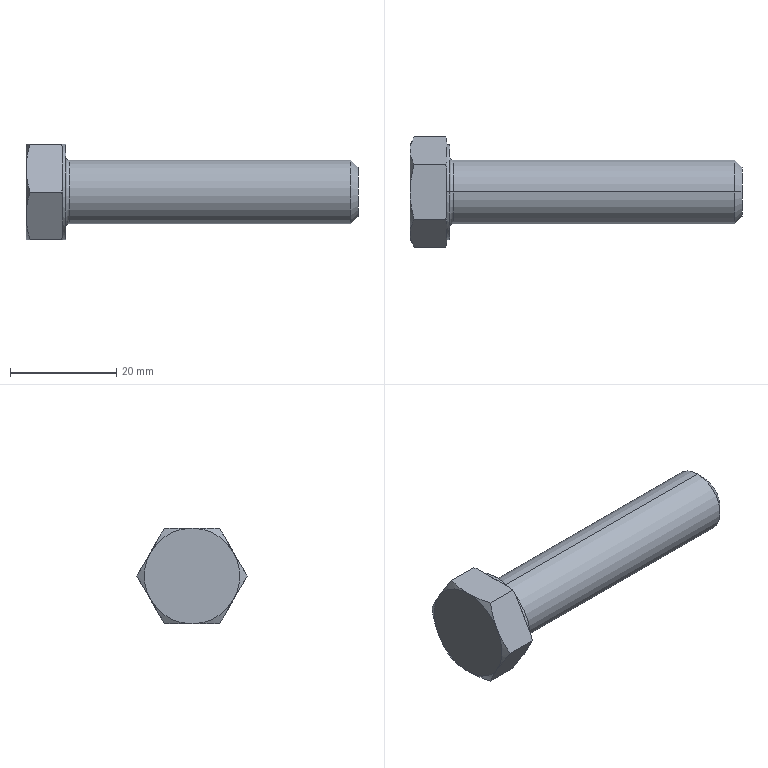Part | SolidWorks | features RevCut 4, Chamfer 1, Extrusion 1, Fillet 1, LPattern 1, Revolution 1 | 1 solid | 35 faces | box 62.5 x 20.785 x 18 mm | volume 8272 mm3 | plane 15 | cone 14 | cylinder 4 | torus 2 | commonest cylinder face diameters 12 x2 18 x2
STEP:
#1=CARTESIAN_POINT('',(8.1,0.,6.));
#2=VERTEX_POINT('',#1);
#3=CARTESIAN_POINT('',(8.1,0.,-6.));
#4=VERTEX_POINT('',#3);
#5=CARTESIAN_POINT('',(8.1,0.,0.));
#6=DIRECTION('',(1.,0.,0.));
#7=DIRECTION('',(0.,0.,-1.));
#8=AXIS2_PLACEMENT_3D('',#5,#6,#7);
#9=CIRCLE('',#8,6.);
#10=EDGE_CURVE('',#2,#4,#9,.T.);
#11=ORIENTED_EDGE('',*,*,#10,.F.);
#12=CARTESIAN_POINT('',(7.5,0.,6.6));
#13=VERTEX_POINT('',#12);
#14=CARTESIAN_POINT('',(8.1,0.,6.6));
#15=DIRECTION('',(0.,1.,0.));
#16=DIRECTION('',(0.,0.,1.));
#17=AXIS2_PLACEMENT_3D('',#14,#15,#16);
#18=CIRCLE('',#17,0.6);
#19=EDGE_CURVE('',#2,#13,#18,.T.);
#20=ORIENTED_EDGE('',*,*,#19,.T.);
#21=CARTESIAN_POINT('',(7.5,0.,-6.6));
#22=VERTEX_POINT('',#21);
#23=CARTESIAN_POINT('',(7.5,0.,0.));
#24=DIRECTION('',(-1.,0.,0.));
#25=DIRECTION('',(0.,0.,-1.));
#26=AXIS2_PLACEMENT_3D('',#23,#24,#25);
#27=CIRCLE('',#26,6.6);
#28=EDGE_CURVE('',#22,#13,#27,.T.);
#29=ORIENTED_EDGE('',*,*,#28,.F.);
#30=CARTESIAN_POINT('',(8.1,0.,-6.6));
#31=DIRECTION('',(0.,-1.,0.));
#32=DIRECTION('',(0.,0.,-1.));
#33=AXIS2_PLACEMENT_3D('',#30,#31,#32);
#34=CIRCLE('',#33,0.6);
#35=EDGE_CURVE('',#4,#22,#34,.T.);
#36=ORIENTED_EDGE('',*,*,#35,.F.);
#37=EDGE_LOOP('',(#11,#20,#29,#36));
#38=FACE_OUTER_BOUND('',#37,.T.);
#39=CARTESIAN_POINT('',(8.1,0.,0.));
#40=DIRECTION('',(1.,0.,0.));
#41=DIRECTION('',(0.,0.,-1.));
#42=AXIS2_PLACEMENT_3D('',#39,#40,#41);
#43=TOROIDAL_SURFACE('',#42,6.6,0.6);
#44=ADVANCED_FACE('',(#38),#43,.F.);
#45=CARTESIAN_POINT('',(62.5,0.,-4.6));
#46=VERTEX_POINT('',#45);
#47=CARTESIAN_POINT('',(62.5,0.,4.6));
#48=VERTEX_POINT('',#47);
#49=CARTESIAN_POINT('',(62.5,0.,0.));
#50=DIRECTION('',(1.,0.,0.));
#51=DIRECTION('',(0.,0.,1.));
#52=AXIS2_PLACEMENT_3D('',#49,#50,#51);
#53=CIRCLE('',#52,4.6);
#54=EDGE_CURVE('',#46,#48,#53,.T.);
#55=ORIENTED_EDGE('',*,*,#54,.F.);
#56=CARTESIAN_POINT('',(61.1,0.,-6.));
#57=VERTEX_POINT('',#56);
#58=CARTESIAN_POINT('',(61.1,0.,-6.));
#59=DIRECTION('',(-0.7071,0.,-0.7071));
#60=VECTOR('',#59,1000.);
#61=LINE('',#58,#60);
#62=EDGE_CURVE('',#46,#57,#61,.T.);
#63=ORIENTED_EDGE('',*,*,#62,.T.);
#64=CARTESIAN_POINT('',(61.1,0.,6.));
#65=VERTEX_POINT('',#64);
#66=CARTESIAN_POINT('',(61.1,0.,0.));
#67=DIRECTION('',(-1.,0.,0.));
#68=DIRECTION('',(0.,0.,1.));
#69=AXIS2_PLACEMENT_3D('',#66,#67,#68);
#70=CIRCLE('',#69,6.);
#71=EDGE_CURVE('',#65,#57,#70,.T.);
#72=ORIENTED_EDGE('',*,*,#71,.F.);
#73=CARTESIAN_POINT('',(61.1,0.,6.));
#74=DIRECTION('',(-0.7071,0.,0.7071));
#75=VECTOR('',#74,1000.);
#76=LINE('',#73,#75);
#77=EDGE_CURVE('',#48,#65,#76,.T.);
#78=ORIENTED_EDGE('',*,*,#77,.F.);
#79=EDGE_LOOP('',(#55,#63,#72,#78));
#80=FACE_OUTER_BOUND('',#79,.T.);
#81=CARTESIAN_POINT('',(61.1,0.,0.));
#82=DIRECTION('',(-1.,0.,0.));
#83=DIRECTION('',(0.,0.,1.));
#84=AXIS2_PLACEMENT_3D('',#81,#82,#83);
#85=CONICAL_SURFACE('',#84,6.,0.7854);
#86=ADVANCED_FACE('',(#80),#85,.T.);
#87=ORIENTED_EDGE('',*,*,#71,.T.);
#88=CARTESIAN_POINT('',(0.,0.,-6.));
#89=DIRECTION('',(-1.,0.,0.));
#90=VECTOR('',#89,1000.);
#91=LINE('',#88,#90);
#92=EDGE_CURVE('',#57,#4,#91,.T.);
#93=ORIENTED_EDGE('',*,*,#92,.T.);
#94=CARTESIAN_POINT('',(8.1,0.,0.));
#95=DIRECTION('',(1.,0.,0.));
#96=DIRECTION('',(0.,0.,-1.));
#97=AXIS2_PLACEMENT_3D('',#94,#95,#96);
#98=CIRCLE('',#97,6.);
#99=EDGE_CURVE('',#4,#2,#98,.T.);
#100=ORIENTED_EDGE('',*,*,#99,.T.);
#101=CARTESIAN_POINT('',(0.,0.,6.));
#102=DIRECTION('',(-1.,0.,0.));
#103=VECTOR('',#102,1000.);
#104=LINE('',#101,#103);
#105=EDGE_CURVE('',#65,#2,#104,.T.);
#106=ORIENTED_EDGE('',*,*,#105,.F.);
#107=EDGE_LOOP('',(#87,#93,#100,#106));
#108=FACE_OUTER_BOUND('',#107,.T.);
#109=CARTESIAN_POINT('',(0.,0.,0.));
#110=DIRECTION('',(-1.,0.,0.));
#111=DIRECTION('',(0.,0.,1.));
#112=AXIS2_PLACEMENT_3D('',#109,#110,#111);
#113=CYLINDRICAL_SURFACE('',#112,6.);
#114=ADVANCED_FACE('',(#108),#113,.T.);
#115=CARTESIAN_POINT('',(7.5,0.,-9.));
#116=VERTEX_POINT('',#115);
#117=CARTESIAN_POINT('',(7.5,0.,9.));
#118=VERTEX_POINT('',#117);
#119=CARTESIAN_POINT('',(7.5,0.,0.));
#120=DIRECTION('',(1.,0.,0.));
#121=DIRECTION('',(0.,0.,-1.));
#122=AXIS2_PLACEMENT_3D('',#119,#120,#121);
#123=CIRCLE('',#122,9.);
#124=EDGE_CURVE('',#116,#118,#123,.T.);
#125=ORIENTED_EDGE('',*,*,#124,.F.);
#126=CARTESIAN_POINT('',(6.9,0.,-9.));
#127=VERTEX_POINT('',#126);
#128=CARTESIAN_POINT('',(0.,0.,-9.));
#129=DIRECTION('',(-1.,0.,0.));
#130=VECTOR('',#129,1000.);
#131=LINE('',#128,#130);
#132=EDGE_CURVE('',#116,#127,#131,.T.);
#133=ORIENTED_EDGE('',*,*,#132,.T.);
#134=CARTESIAN_POINT('',(6.9,7.794,-4.5));
#135=VERTEX_POINT('',#134);
#136=CARTESIAN_POINT('',(6.9,0.,0.));
#137=DIRECTION('',(-1.,0.,0.));
#138=DIRECTION('',(0.,0.,1.));
#139=AXIS2_PLACEMENT_3D('',#136,#137,#138);
#140=CIRCLE('',#139,9.);
#141=EDGE_CURVE('',#135,#127,#140,.T.);
#142=ORIENTED_EDGE('',*,*,#141,.F.);
#143=CARTESIAN_POINT('',(6.9,7.794,4.5));
#144=VERTEX_POINT('',#143);
#145=CARTESIAN_POINT('',(6.9,0.,0.));
#146=DIRECTION('',(-1.,0.,0.));
#147=DIRECTION('',(0.,0.,1.));
#148=AXIS2_PLACEMENT_3D('',#145,#146,#147);
#149=CIRCLE('',#148,9.);
#150=EDGE_CURVE('',#144,#135,#149,.T.);
#151=ORIENTED_EDGE('',*,*,#150,.F.);
#152=CARTESIAN_POINT('',(6.9,0.,9.));
#153=VERTEX_POINT('',#152);
#154=CARTESIAN_POINT('',(6.9,0.,0.));
#155=DIRECTION('',(-1.,0.,0.));
#156=DIRECTION('',(0.,0.,1.));
#157=AXIS2_PLACEMENT_3D('',#154,#155,#156);
#158=CIRCLE('',#157,9.);
#159=EDGE_CURVE('',#153,#144,#158,.T.);
#160=ORIENTED_EDGE('',*,*,#159,.F.);
#161=CARTESIAN_POINT('',(0.,0.,9.));
#162=DIRECTION('',(-1.,0.,0.));
#163=VECTOR('',#162,1000.);
#164=LINE('',#161,#163);
#165=EDGE_CURVE('',#118,#153,#164,.T.);
#166=ORIENTED_EDGE('',*,*,#165,.F.);
#167=EDGE_LOOP('',(#125,#133,#142,#151,#160,#166));
#168=FACE_OUTER_BOUND('',#167,.T.);
#169=CARTESIAN_POINT('',(0.,0.,0.));
#170=DIRECTION('',(-1.,0.,0.));
#171=DIRECTION('',(0.,0.,1.));
#172=AXIS2_PLACEMENT_3D('',#169,#170,#171);
#173=CYLINDRICAL_SURFACE('',#172,9.);
#174=ADVANCED_FACE('',(#168),#173,.T.);
#175=CARTESIAN_POINT('',(6.9,5.57,-8.352));
#176=VERTEX_POINT('',#175);
#177=CARTESIAN_POINT('',(6.9,5.196,-9.));
#178=DIRECTION('',(0.,0.5,0.866));
#179=VECTOR('',#178,1000.);
#180=LINE('',#177,#179);
#181=EDGE_CURVE('',#176,#135,#180,.T.);
#182=ORIENTED_EDGE('',*,*,#181,.F.);
#183=CARTESIAN_POINT('',(6.696,5.196,-9.));
#184=VERTEX_POINT('',#183);
#185=CARTESIAN_POINT('',(6.696,5.196,-9.));
#186=CARTESIAN_POINT('',(6.768,5.321,-8.785));
#187=CARTESIAN_POINT('',(6.836,5.445,-8.569));
#188=CARTESIAN_POINT('',(6.9,5.57,-8.352));
#189=B_SPLINE_CURVE_WITH_KNOTS('',3,(#185,#186,#187,#188),.UNSPECIFIED.,.F.,.F.,(4,4),(0.000000238,0.0007696),.UNSPECIFIED.);
#190=EDGE_CURVE('',#184,#176,#189,.T.);
#191=ORIENTED_EDGE('',*,*,#190,.F.);
#192=CARTESIAN_POINT('',(0.8038,5.196,-9.));
#193=VERTEX_POINT('',#192);
#194=CARTESIAN_POINT('',(7.5,5.196,-9.));
#195=DIRECTION('',(-1.,0.,0.));
#196=VECTOR('',#195,1000.);
#197=LINE('',#194,#196);
#198=EDGE_CURVE('',#184,#193,#197,.T.);
#199=ORIENTED_EDGE('',*,*,#198,.T.);
#200=CARTESIAN_POINT('',(0.,7.794,-4.5));
#201=VERTEX_POINT('',#200);
#202=CARTESIAN_POINT('',(0.,7.794,-4.5));
#203=CARTESIAN_POINT('',(0.,7.574,-4.882));
#204=CARTESIAN_POINT('',(0.019,7.352,-5.266));
#205=CARTESIAN_POINT('',(0.09253,6.914,-6.024));
#206=CARTESIAN_POINT('',(0.147,6.697,-6.401));
#207=CARTESIAN_POINT('',(0.357,6.048,-7.525));
#208=CARTESIAN_POINT('',(0.5591,5.62,-8.266));
#209=CARTESIAN_POINT('',(0.8038,5.196,-9.));
#210=B_SPLINE_CURVE_WITH_KNOTS('',3,(#202,#203,#204,#205,#206,#207,#208,#209),.UNSPECIFIED.,.F.,.F.,(4,2,2,4),(0.005258,0.006567,0.007877,0.0105),.UNSPECIFIED.);
#211=EDGE_CURVE('',#201,#193,#210,.T.);
#212=ORIENTED_EDGE('',*,*,#211,.F.);
#213=CARTESIAN_POINT('',(0.8038,10.392,0.));
#214=VERTEX_POINT('',#213);
#215=CARTESIAN_POINT('',(0.8038,10.392,0.));
#216=CARTESIAN_POINT('',(0.5585,9.967,-0.7361));
#217=CARTESIAN_POINT('',(0.3563,9.539,-1.478));
#218=CARTESIAN_POINT('',(0.07661,8.674,-2.976));
#219=CARTESIAN_POINT('',(0.,8.237,-3.733));
#220=CARTESIAN_POINT('',(0.,7.794,-4.5));
#221=B_SPLINE_CURVE_WITH_KNOTS('',3,(#215,#216,#217,#218,#219,#220),.UNSPECIFIED.,.F.,.F.,(4,2,4),(0.000000238,0.002629,0.005258),.UNSPECIFIED.);
#222=EDGE_CURVE('',#214,#201,#221,.T.);
#223=ORIENTED_EDGE('',*,*,#222,.F.);
#224=CARTESIAN_POINT('',(6.696,10.392,0.));
#225=VERTEX_POINT('',#224);
#226=CARTESIAN_POINT('',(7.5,10.392,0.));
#227=DIRECTION('',(-1.,0.,0.));
#228=VECTOR('',#227,1000.);
#229=LINE('',#226,#228);
#230=EDGE_CURVE('',#225,#214,#229,.T.);
#231=ORIENTED_EDGE('',*,*,#230,.F.);
#232=CARTESIAN_POINT('',(6.9,10.018,-0.6478));
#233=VERTEX_POINT('',#232);
#234=CARTESIAN_POINT('',(6.9,10.018,-0.6478));
#235=CARTESIAN_POINT('',(6.836,10.143,-0.4313));
#236=CARTESIAN_POINT('',(6.768,10.268,-0.2154));
#237=CARTESIAN_POINT('',(6.696,10.392,0.));
#238=B_SPLINE_CURVE_WITH_KNOTS('',3,(#234,#235,#236,#237),.UNSPECIFIED.,.F.,.F.,(4,4),(0.009728,0.0105),.UNSPECIFIED.);
#239=EDGE_CURVE('',#233,#225,#238,.T.);
#240=ORIENTED_EDGE('',*,*,#239,.F.);
#241=CARTESIAN_POINT('',(6.9,5.196,-9.));
#242=DIRECTION('',(0.,0.5,0.866));
#243=VECTOR('',#242,1000.);
#244=LINE('',#241,#243);
#245=EDGE_CURVE('',#135,#233,#244,.T.);
#246=ORIENTED_EDGE('',*,*,#245,.F.);
#247=EDGE_LOOP('',(#182,#191,#199,#212,#223,#231,#240,#246));
#248=FACE_OUTER_BOUND('',#247,.T.);
#249=CARTESIAN_POINT('',(7.5,5.196,-9.));
#250=DIRECTION('',(0.,-0.866,0.5));
#251=DIRECTION('',(0.,-0.5,-0.866));
#252=AXIS2_PLACEMENT_3D('',#249,#250,#251);
#253=PLANE('',#252);
#254=ADVANCED_FACE('',(#248),#253,.F.);
#255=CARTESIAN_POINT('',(6.9,10.018,0.6478));
#256=VERTEX_POINT('',#255);
#257=CARTESIAN_POINT('',(6.9,10.392,0.));
#258=DIRECTION('',(0.,-0.5,0.866));
#259=VECTOR('',#258,1000.);
#260=LINE('',#257,#259);
#261=EDGE_CURVE('',#256,#144,#260,.T.);
#262=ORIENTED_EDGE('',*,*,#261,.F.);
#263=CARTESIAN_POINT('',(6.696,10.392,0.));
#264=CARTESIAN_POINT('',(6.768,10.268,0.2154));
#265=CARTESIAN_POINT('',(6.836,10.143,0.4314));
#266=CARTESIAN_POINT('',(6.9,10.018,0.6478));
#267=B_SPLINE_CURVE_WITH_KNOTS('',3,(#263,#264,#265,#266),.UNSPECIFIED.,.F.,.F.,(4,4),(0.000000238,0.0007696),.UNSPECIFIED.);
#268=EDGE_CURVE('',#225,#256,#267,.T.);
#269=ORIENTED_EDGE('',*,*,#268,.F.);
#270=ORIENTED_EDGE('',*,*,#230,.T.);
#271=CARTESIAN_POINT('',(0.,7.794,4.5));
#272=VERTEX_POINT('',#271);
#273=CARTESIAN_POINT('',(0.,7.794,4.5));
#274=CARTESIAN_POINT('',(0.,8.015,4.118));
#275=CARTESIAN_POINT('',(0.019,8.236,3.734));
#276=CARTESIAN_POINT('',(0.09253,8.674,2.976));
#277=CARTESIAN_POINT('',(0.147,8.892,2.599));
#278=CARTESIAN_POINT('',(0.357,9.541,1.475));
#279=CARTESIAN_POINT('',(0.5591,9.968,0.7343));
#280=CARTESIAN_POINT('',(0.8038,10.392,0.));
#281=B_SPLINE_CURVE_WITH_KNOTS('',3,(#273,#274,#275,#276,#277,#278,#279,#280),.UNSPECIFIED.,.F.,.F.,(4,2,2,4),(0.005258,0.006567,0.007877,0.0105),.UNSPECIFIED.);
#282=EDGE_CURVE('',#272,#214,#281,.T.);
#283=ORIENTED_EDGE('',*,*,#282,.F.);
#284=CARTESIAN_POINT('',(0.8038,5.196,9.));
#285=VERTEX_POINT('',#284);
#286=CARTESIAN_POINT('',(0.8038,5.196,9.));
#287=CARTESIAN_POINT('',(0.5585,5.621,8.264));
#288=CARTESIAN_POINT('',(0.3563,6.049,7.522));
#289=CARTESIAN_POINT('',(0.07661,6.914,6.024));
#290=CARTESIAN_POINT('',(0.,7.352,5.267));
#291=CARTESIAN_POINT('',(0.,7.794,4.5));
#292=B_SPLINE_CURVE_WITH_KNOTS('',3,(#286,#287,#288,#289,#290,#291),.UNSPECIFIED.,.F.,.F.,(4,2,4),(0.000000238,0.002629,0.005258),.UNSPECIFIED.);
#293=EDGE_CURVE('',#285,#272,#292,.T.);
#294=ORIENTED_EDGE('',*,*,#293,.F.);
#295=CARTESIAN_POINT('',(6.696,5.196,9.));
#296=VERTEX_POINT('',#295);
#297=CARTESIAN_POINT('',(7.5,5.196,9.));
#298=DIRECTION('',(-1.,0.,0.));
#299=VECTOR('',#298,1000.);
#300=LINE('',#297,#299);
#301=EDGE_CURVE('',#296,#285,#300,.T.);
#302=ORIENTED_EDGE('',*,*,#301,.F.);
#303=CARTESIAN_POINT('',(6.9,5.57,8.352));
#304=VERTEX_POINT('',#303);
#305=CARTESIAN_POINT('',(6.9,5.57,8.352));
#306=CARTESIAN_POINT('',(6.836,5.445,8.569));
#307=CARTESIAN_POINT('',(6.768,5.32,8.785));
#308=CARTESIAN_POINT('',(6.696,5.196,9.));
#309=B_SPLINE_CURVE_WITH_KNOTS('',3,(#305,#306,#307,#308),.UNSPECIFIED.,.F.,.F.,(4,4),(0.009728,0.0105),.UNSPECIFIED.);
#310=EDGE_CURVE('',#304,#296,#309,.T.);
#311=ORIENTED_EDGE('',*,*,#310,.F.);
#312=CARTESIAN_POINT('',(6.9,10.392,0.));
#313=DIRECTION('',(0.,-0.5,0.866));
#314=VECTOR('',#313,1000.);
#315=LINE('',#312,#314);
#316=EDGE_CURVE('',#144,#304,#315,.T.);
#317=ORIENTED_EDGE('',*,*,#316,.F.);
#318=EDGE_LOOP('',(#262,#269,#270,#283,#294,#302,#311,#317));
#319=FACE_OUTER_BOUND('',#318,.T.);
#320=CARTESIAN_POINT('',(7.5,10.392,0.));
#321=DIRECTION('',(0.,-0.866,-0.5));
#322=DIRECTION('',(0.,0.5,-0.866));
#323=AXIS2_PLACEMENT_3D('',#320,#321,#322);
#324=PLANE('',#323);
#325=ADVANCED_FACE('',(#319),#324,.F.);
#326=CARTESIAN_POINT('',(6.9,4.448,9.));
#327=VERTEX_POINT('',#326);
#328=CARTESIAN_POINT('',(6.9,5.196,9.));
#329=DIRECTION('',(0.,-1.,0.));
#330=VECTOR('',#329,1000.);
#331=LINE('',#328,#330);
#332=EDGE_CURVE('',#327,#153,#331,.T.);
#333=ORIENTED_EDGE('',*,*,#332,.F.);
#334=CARTESIAN_POINT('',(6.696,5.196,9.));
#335=CARTESIAN_POINT('',(6.768,4.948,9.));
#336=CARTESIAN_POINT('',(6.836,4.698,9.));
#337=CARTESIAN_POINT('',(6.9,4.448,9.));
#338=B_SPLINE_CURVE_WITH_KNOTS('',3,(#334,#335,#336,#337),.UNSPECIFIED.,.F.,.F.,(4,4),(0.02519,0.02597),.UNSPECIFIED.);
#339=EDGE_CURVE('',#296,#327,#338,.T.);
#340=ORIENTED_EDGE('',*,*,#339,.F.);
#341=ORIENTED_EDGE('',*,*,#301,.T.);
#342=CARTESIAN_POINT('',(0.,0.,9.));
#343=VERTEX_POINT('',#342);
#344=CARTESIAN_POINT('',(0.,0.,9.));
#345=CARTESIAN_POINT('',(0.,0.4401,9.));
#346=CARTESIAN_POINT('',(0.01885,0.8832,9.));
#347=CARTESIAN_POINT('',(0.09319,1.767,9.));
#348=CARTESIAN_POINT('',(0.1482,2.204,9.));
#349=CARTESIAN_POINT('',(0.3593,3.505,9.));
#350=CARTESIAN_POINT('',(0.5612,4.356,9.));
#351=CARTESIAN_POINT('',(0.8038,5.196,9.));
#352=B_SPLINE_CURVE_WITH_KNOTS('',3,(#344,#345,#346,#347,#348,#349,#350,#351),.UNSPECIFIED.,.F.,.F.,(4,2,2,4),(0.01498,0.0163,0.01761,0.02025),.UNSPECIFIED.);
#353=EDGE_CURVE('',#343,#285,#352,.T.);
#354=ORIENTED_EDGE('',*,*,#353,.F.);
#355=CARTESIAN_POINT('',(0.8038,-5.196,9.));
#356=VERTEX_POINT('',#355);
#357=CARTESIAN_POINT('',(0.8038,-5.196,9.));
#358=CARTESIAN_POINT('',(0.5595,-4.35,9.));
#359=CARTESIAN_POINT('',(0.3552,-3.485,9.));
#360=CARTESIAN_POINT('',(0.07569,-1.752,9.));
#361=CARTESIAN_POINT('',(0.,-0.8794,9.));
#362=CARTESIAN_POINT('',(0.,0.,9.));
#363=B_SPLINE_CURVE_WITH_KNOTS('',3,(#357,#358,#359,#360,#361,#362),.UNSPECIFIED.,.F.,.F.,(4,2,4),(0.00972,0.01235,0.01498),.UNSPECIFIED.);
#364=EDGE_CURVE('',#356,#343,#363,.T.);
#365=ORIENTED_EDGE('',*,*,#364,.F.);
#366=CARTESIAN_POINT('',(6.696,-5.196,9.));
#367=VERTEX_POINT('',#366);
#368=CARTESIAN_POINT('',(7.5,-5.196,9.));
#369=DIRECTION('',(-1.,0.,0.));
#370=VECTOR('',#369,1000.);
#371=LINE('',#368,#370);
#372=EDGE_CURVE('',#367,#356,#371,.T.);
#373=ORIENTED_EDGE('',*,*,#372,.F.);
#374=CARTESIAN_POINT('',(6.9,-4.448,9.));
#375=VERTEX_POINT('',#374);
#376=CARTESIAN_POINT('',(6.9,-4.448,9.));
#377=CARTESIAN_POINT('',(6.836,-4.699,9.));
#378=CARTESIAN_POINT('',(6.768,-4.948,9.));
#379=CARTESIAN_POINT('',(6.696,-5.196,9.));
#380=B_SPLINE_CURVE_WITH_KNOTS('',3,(#376,#377,#378,#379),.UNSPECIFIED.,.F.,.F.,(4,4),(0.03494,0.03571),.UNSPECIFIED.);
#381=EDGE_CURVE('',#375,#367,#380,.T.);
#382=ORIENTED_EDGE('',*,*,#381,.F.);
#383=CARTESIAN_POINT('',(6.9,5.196,9.));
#384=DIRECTION('',(0.,-1.,0.));
#385=VECTOR('',#384,1000.);
#386=LINE('',#383,#385);
#387=EDGE_CURVE('',#153,#375,#386,.T.);
#388=ORIENTED_EDGE('',*,*,#387,.F.);
#389=EDGE_LOOP('',(#333,#340,#341,#354,#365,#373,#382,#388));
#390=FACE_OUTER_BOUND('',#389,.T.);
#391=CARTESIAN_POINT('',(7.5,5.196,9.));
#392=DIRECTION('',(0.,0.,-1.));
#393=DIRECTION('',(-1.,0.,0.));
#394=AXIS2_PLACEMENT_3D('',#391,#392,#393);
#395=PLANE('',#394);
#396=ADVANCED_FACE('',(#390),#395,.F.);
#397=CARTESIAN_POINT('',(6.9,-5.57,8.352));
#398=VERTEX_POINT('',#397);
#399=CARTESIAN_POINT('',(6.9,-7.794,4.5));
#400=VERTEX_POINT('',#399);
#401=CARTESIAN_POINT('',(6.9,-10.392,0.));
#402=DIRECTION('',(0.,-0.5,-0.866));
#403=VECTOR('',#402,1000.);
#404=LINE('',#401,#403);
#405=EDGE_CURVE('',#398,#400,#404,.T.);
#406=ORIENTED_EDGE('',*,*,#405,.F.);
#407=CARTESIAN_POINT('',(6.696,-5.196,9.));
#408=CARTESIAN_POINT('',(6.768,-5.321,8.785));
#409=CARTESIAN_POINT('',(6.836,-5.445,8.569));
#410=CARTESIAN_POINT('',(6.9,-5.57,8.352));
#411=B_SPLINE_CURVE_WITH_KNOTS('',3,(#407,#408,#409,#410),.UNSPECIFIED.,.F.,.F.,(4,4),(0.000000238,0.0007696),.UNSPECIFIED.);
#412=EDGE_CURVE('',#367,#398,#411,.T.);
#413=ORIENTED_EDGE('',*,*,#412,.F.);
#414=ORIENTED_EDGE('',*,*,#372,.T.);
#415=CARTESIAN_POINT('',(0.,-7.794,4.5));
#416=VERTEX_POINT('',#415);
#417=CARTESIAN_POINT('',(0.,-7.794,4.5));
#418=CARTESIAN_POINT('',(0.,-7.574,4.882));
#419=CARTESIAN_POINT('',(0.019,-7.352,5.266));
#420=CARTESIAN_POINT('',(0.09253,-6.914,6.024));
#421=CARTESIAN_POINT('',(0.147,-6.697,6.401));
#422=CARTESIAN_POINT('',(0.357,-6.048,7.525));
#423=CARTESIAN_POINT('',(0.5591,-5.62,8.266));
#424=CARTESIAN_POINT('',(0.8038,-5.196,9.));
#425=B_SPLINE_CURVE_WITH_KNOTS('',3,(#417,#418,#419,#420,#421,#422,#423,#424),.UNSPECIFIED.,.F.,.F.,(4,2,2,4),(0.005258,0.006567,0.007877,0.0105),.UNSPECIFIED.);
#426=EDGE_CURVE('',#416,#356,#425,.T.);
#427=ORIENTED_EDGE('',*,*,#426,.F.);
#428=CARTESIAN_POINT('',(0.8038,-10.392,0.));
#429=VERTEX_POINT('',#428);
#430=CARTESIAN_POINT('',(0.8038,-10.392,0.));
#431=CARTESIAN_POINT('',(0.5585,-9.967,0.7361));
#432=CARTESIAN_POINT('',(0.3563,-9.539,1.478));
#433=CARTESIAN_POINT('',(0.07661,-8.674,2.976));
#434=CARTESIAN_POINT('',(0.,-8.237,3.733));
#435=CARTESIAN_POINT('',(0.,-7.794,4.5));
#436=B_SPLINE_CURVE_WITH_KNOTS('',3,(#430,#431,#432,#433,#434,#435),.UNSPECIFIED.,.F.,.F.,(4,2,4),(0.000000238,0.002629,0.005258),.UNSPECIFIED.);
#437=EDGE_CURVE('',#429,#416,#436,.T.);
#438=ORIENTED_EDGE('',*,*,#437,.F.);
#439=CARTESIAN_POINT('',(6.696,-10.392,0.));
#440=VERTEX_POINT('',#439);
#441=CARTESIAN_POINT('',(7.5,-10.392,0.));
#442=DIRECTION('',(-1.,0.,0.));
#443=VECTOR('',#442,1000.);
#444=LINE('',#441,#443);
#445=EDGE_CURVE('',#440,#429,#444,.T.);
#446=ORIENTED_EDGE('',*,*,#445,.F.);
#447=CARTESIAN_POINT('',(6.9,-10.018,0.6478));
#448=VERTEX_POINT('',#447);
#449=CARTESIAN_POINT('',(6.9,-10.018,0.6478));
#450=CARTESIAN_POINT('',(6.836,-10.143,0.4313));
#451=CARTESIAN_POINT('',(6.768,-10.268,0.2154));
#452=CARTESIAN_POINT('',(6.696,-10.392,0.));
#453=B_SPLINE_CURVE_WITH_KNOTS('',3,(#449,#450,#451,#452),.UNSPECIFIED.,.F.,.F.,(4,4),(0.009728,0.0105),.UNSPECIFIED.);
#454=EDGE_CURVE('',#448,#440,#453,.T.);
#455=ORIENTED_EDGE('',*,*,#454,.F.);
#456=CARTESIAN_POINT('',(6.9,-10.392,0.));
#457=DIRECTION('',(0.,-0.5,-0.866));
#458=VECTOR('',#457,1000.);
#459=LINE('',#456,#458);
#460=EDGE_CURVE('',#400,#448,#459,.T.);
#461=ORIENTED_EDGE('',*,*,#460,.F.);
#462=EDGE_LOOP('',(#406,#413,#414,#427,#438,#446,#455,#461));
#463=FACE_OUTER_BOUND('',#462,.T.);
#464=CARTESIAN_POINT('',(7.5,-10.392,0.));
#465=DIRECTION('',(0.,0.866,-0.5));
#466=DIRECTION('',(0.,0.5,0.866));
#467=AXIS2_PLACEMENT_3D('',#464,#465,#466);
#468=PLANE('',#467);
#469=ADVANCED_FACE('',(#463),#468,.F.);
#470=CARTESIAN_POINT('',(6.9,-10.018,-0.6478));
#471=VERTEX_POINT('',#470);
#472=CARTESIAN_POINT('',(6.9,-7.794,-4.5));
#473=VERTEX_POINT('',#472);
#474=CARTESIAN_POINT('',(6.9,-5.196,-9.));
#475=DIRECTION('',(0.,0.5,-0.866));
#476=VECTOR('',#475,1000.);
#477=LINE('',#474,#476);
#478=EDGE_CURVE('',#471,#473,#477,.T.);
#479=ORIENTED_EDGE('',*,*,#478,.F.);
#480=CARTESIAN_POINT('',(6.696,-10.392,0.));
#481=CARTESIAN_POINT('',(6.768,-10.268,-0.2154));
#482=CARTESIAN_POINT('',(6.836,-10.143,-0.4314));
#483=CARTESIAN_POINT('',(6.9,-10.018,-0.6478));
#484=B_SPLINE_CURVE_WITH_KNOTS('',3,(#480,#481,#482,#483),.UNSPECIFIED.,.F.,.F.,(4,4),(0.000000238,0.0007696),.UNSPECIFIED.);
#485=EDGE_CURVE('',#440,#471,#484,.T.);
#486=ORIENTED_EDGE('',*,*,#485,.F.);
#487=ORIENTED_EDGE('',*,*,#445,.T.);
#488=CARTESIAN_POINT('',(0.,-7.794,-4.5));
#489=VERTEX_POINT('',#488);
#490=CARTESIAN_POINT('',(0.,-7.794,-4.5));
#491=CARTESIAN_POINT('',(0.,-8.015,-4.118));
#492=CARTESIAN_POINT('',(0.019,-8.236,-3.734));
#493=CARTESIAN_POINT('',(0.09253,-8.674,-2.976));
#494=CARTESIAN_POINT('',(0.147,-8.892,-2.599));
#495=CARTESIAN_POINT('',(0.357,-9.541,-1.475));
#496=CARTESIAN_POINT('',(0.5591,-9.968,-0.7343));
#497=CARTESIAN_POINT('',(0.8038,-10.392,0.));
#498=B_SPLINE_CURVE_WITH_KNOTS('',3,(#490,#491,#492,#493,#494,#495,#496,#497),.UNSPECIFIED.,.F.,.F.,(4,2,2,4),(0.005258,0.006567,0.007877,0.0105),.UNSPECIFIED.);
#499=EDGE_CURVE('',#489,#429,#498,.T.);
#500=ORIENTED_EDGE('',*,*,#499,.F.);
#501=CARTESIAN_POINT('',(0.8038,-5.196,-9.));
#502=VERTEX_POINT('',#501);
#503=CARTESIAN_POINT('',(0.8038,-5.196,-9.));
#504=CARTESIAN_POINT('',(0.5585,-5.621,-8.264));
#505=CARTESIAN_POINT('',(0.3563,-6.049,-7.522));
#506=CARTESIAN_POINT('',(0.07661,-6.914,-6.024));
#507=CARTESIAN_POINT('',(0.,-7.352,-5.267));
#508=CARTESIAN_POINT('',(0.,-7.794,-4.5));
#509=B_SPLINE_CURVE_WITH_KNOTS('',3,(#503,#504,#505,#506,#507,#508),.UNSPECIFIED.,.F.,.F.,(4,2,4),(0.000000238,0.002629,0.005258),.UNSPECIFIED.);
#510=EDGE_CURVE('',#502,#489,#509,.T.);
#511=ORIENTED_EDGE('',*,*,#510,.F.);
#512=CARTESIAN_POINT('',(6.696,-5.196,-9.));
#513=VERTEX_POINT('',#512);
#514=CARTESIAN_POINT('',(7.5,-5.196,-9.));
#515=DIRECTION('',(-1.,0.,0.));
#516=VECTOR('',#515,1000.);
#517=LINE('',#514,#516);
#518=EDGE_CURVE('',#513,#502,#517,.T.);
#519=ORIENTED_EDGE('',*,*,#518,.F.);
#520=CARTESIAN_POINT('',(6.9,-5.57,-8.352));
#521=VERTEX_POINT('',#520);
#522=CARTESIAN_POINT('',(6.9,-5.57,-8.352));
#523=CARTESIAN_POINT('',(6.836,-5.445,-8.569));
#524=CARTESIAN_POINT('',(6.768,-5.32,-8.785));
#525=CARTESIAN_POINT('',(6.696,-5.196,-9.));
#526=B_SPLINE_CURVE_WITH_KNOTS('',3,(#522,#523,#524,#525),.UNSPECIFIED.,.F.,.F.,(4,4),(0.009728,0.0105),.UNSPECIFIED.);
#527=EDGE_CURVE('',#521,#513,#526,.T.);
#528=ORIENTED_EDGE('',*,*,#527,.F.);
#529=CARTESIAN_POINT('',(6.9,-5.196,-9.));
#530=DIRECTION('',(0.,0.5,-0.866));
#531=VECTOR('',#530,1000.);
#532=LINE('',#529,#531);
#533=EDGE_CURVE('',#473,#521,#532,.T.);
#534=ORIENTED_EDGE('',*,*,#533,.F.);
#535=EDGE_LOOP('',(#479,#486,#487,#500,#511,#519,#528,#534));
#536=FACE_OUTER_BOUND('',#535,.T.);
#537=CARTESIAN_POINT('',(7.5,-5.196,-9.));
#538=DIRECTION('',(0.,0.866,0.5));
#539=DIRECTION('',(0.,-0.5,0.866));
#540=AXIS2_PLACEMENT_3D('',#537,#538,#539);
#541=PLANE('',#540);
#542=ADVANCED_FACE('',(#536),#541,.F.);
#543=CARTESIAN_POINT('',(6.9,-4.448,-9.));
#544=VERTEX_POINT('',#543);
#545=CARTESIAN_POINT('',(6.9,5.196,-9.));
#546=DIRECTION('',(0.,1.,0.));
#547=VECTOR('',#546,1000.);
#548=LINE('',#545,#547);
#549=EDGE_CURVE('',#544,#127,#548,.T.);
#550=ORIENTED_EDGE('',*,*,#549,.F.);
#551=CARTESIAN_POINT('',(6.696,-5.196,-9.));
#552=CARTESIAN_POINT('',(6.768,-4.948,-9.));
#553=CARTESIAN_POINT('',(6.836,-4.699,-9.));
#554=CARTESIAN_POINT('',(6.9,-4.448,-9.));
#555=B_SPLINE_CURVE_WITH_KNOTS('',3,(#551,#552,#553,#554),.UNSPECIFIED.,.F.,.F.,(4,4),(0.00972,0.01049),.UNSPECIFIED.);
#556=EDGE_CURVE('',#513,#544,#555,.T.);
#557=ORIENTED_EDGE('',*,*,#556,.F.);
#558=ORIENTED_EDGE('',*,*,#518,.T.);
#559=CARTESIAN_POINT('',(0.,0.,-9.));
#560=VERTEX_POINT('',#559);
#561=CARTESIAN_POINT('',(0.,0.,-9.));
#562=CARTESIAN_POINT('',(0.,-0.8794,-9.));
#563=CARTESIAN_POINT('',(0.07569,-1.752,-9.));
#564=CARTESIAN_POINT('',(0.3552,-3.485,-9.));
#565=CARTESIAN_POINT('',(0.5595,-4.35,-9.));
#566=CARTESIAN_POINT('',(0.8038,-5.196,-9.));
#567=B_SPLINE_CURVE_WITH_KNOTS('',3,(#561,#562,#563,#564,#565,#566),.UNSPECIFIED.,.F.,.F.,(4,2,4),(0.03045,0.03308,0.03571),.UNSPECIFIED.);
#568=EDGE_CURVE('',#560,#502,#567,.T.);
#569=ORIENTED_EDGE('',*,*,#568,.F.);
#570=CARTESIAN_POINT('',(0.8038,5.196,-9.));
#571=CARTESIAN_POINT('',(0.5612,4.356,-9.));
#572=CARTESIAN_POINT('',(0.3593,3.505,-9.));
#573=CARTESIAN_POINT('',(0.1482,2.204,-9.));
#574=CARTESIAN_POINT('',(0.09319,1.767,-9.));
#575=CARTESIAN_POINT('',(0.01885,0.8832,-9.));
#576=CARTESIAN_POINT('',(0.,0.4401,-9.));
#577=CARTESIAN_POINT('',(0.,0.,-9.));
#578=B_SPLINE_CURVE_WITH_KNOTS('',3,(#570,#571,#572,#573,#574,#575,#576,#577),.UNSPECIFIED.,.F.,.F.,(4,2,2,4),(0.02519,0.02782,0.02914,0.03045),.UNSPECIFIED.);
#579=EDGE_CURVE('',#193,#560,#578,.T.);
#580=ORIENTED_EDGE('',*,*,#579,.F.);
#581=ORIENTED_EDGE('',*,*,#198,.F.);
#582=CARTESIAN_POINT('',(6.9,4.448,-9.));
#583=VERTEX_POINT('',#582);
#584=CARTESIAN_POINT('',(6.9,4.448,-9.));
#585=CARTESIAN_POINT('',(6.836,4.698,-9.));
#586=CARTESIAN_POINT('',(6.768,4.948,-9.));
#587=CARTESIAN_POINT('',(6.696,5.196,-9.));
#588=B_SPLINE_CURVE_WITH_KNOTS('',3,(#584,#585,#586,#587),.UNSPECIFIED.,.F.,.F.,(4,4),(0.01947,0.02025),.UNSPECIFIED.);
#589=EDGE_CURVE('',#583,#184,#588,.T.);
#590=ORIENTED_EDGE('',*,*,#589,.F.);
#591=CARTESIAN_POINT('',(6.9,5.196,-9.));
#592=DIRECTION('',(0.,1.,0.));
#593=VECTOR('',#592,1000.);
#594=LINE('',#591,#593);
#595=EDGE_CURVE('',#127,#583,#594,.T.);
#596=ORIENTED_EDGE('',*,*,#595,.F.);
#597=EDGE_LOOP('',(#550,#557,#558,#569,#580,#581,#590,#596));
#598=FACE_OUTER_BOUND('',#597,.T.);
#599=CARTESIAN_POINT('',(7.5,5.196,-9.));
#600=DIRECTION('',(0.,0.,1.));
#601=DIRECTION('',(1.,0.,0.));
#602=AXIS2_PLACEMENT_3D('',#599,#600,#601);
#603=PLANE('',#602);
#604=ADVANCED_FACE('',(#598),#603,.F.);
#605=ORIENTED_EDGE('',*,*,#556,.T.);
#606=CARTESIAN_POINT('',(6.9,0.,0.));
#607=DIRECTION('',(-1.,0.,0.));
#608=DIRECTION('',(0.,0.,-1.));
#609=AXIS2_PLACEMENT_3D('',#606,#607,#608);
#610=CIRCLE('',#609,10.039);
#611=EDGE_CURVE('',#544,#521,#610,.T.);
#612=ORIENTED_EDGE('',*,*,#611,.T.);
#613=ORIENTED_EDGE('',*,*,#527,.T.);
#614=EDGE_LOOP('',(#605,#612,#613));
#615=FACE_OUTER_BOUND('',#614,.T.);
#616=CARTESIAN_POINT('',(3.809,0.,0.));
#617=DIRECTION('',(-1.,0.,0.));
#618=DIRECTION('',(0.,0.,1.));
#619=AXIS2_PLACEMENT_3D('',#616,#617,#618);
#620=CONICAL_SURFACE('',#619,15.392,1.047);
#621=ADVANCED_FACE('',(#615),#620,.T.);
#622=ORIENTED_EDGE('',*,*,#485,.T.);
#623=CARTESIAN_POINT('',(6.9,0.,0.));
#624=DIRECTION('',(-1.,0.,0.));
#625=DIRECTION('',(0.,0.,-1.));
#626=AXIS2_PLACEMENT_3D('',#623,#624,#625);
#627=CIRCLE('',#626,10.039);
#628=EDGE_CURVE('',#471,#448,#627,.T.);
#629=ORIENTED_EDGE('',*,*,#628,.T.);
#630=ORIENTED_EDGE('',*,*,#454,.T.);
#631=EDGE_LOOP('',(#622,#629,#630));
#632=FACE_OUTER_BOUND('',#631,.T.);
#633=CARTESIAN_POINT('',(3.809,0.,0.));
#634=DIRECTION('',(-1.,0.,0.));
#635=DIRECTION('',(0.,0.,1.));
#636=AXIS2_PLACEMENT_3D('',#633,#634,#635);
#637=CONICAL_SURFACE('',#636,15.392,1.047);
#638=ADVANCED_FACE('',(#632),#637,.T.);
#639=ORIENTED_EDGE('',*,*,#412,.T.);
#640=CARTESIAN_POINT('',(6.9,0.,0.));
#641=DIRECTION('',(-1.,0.,0.));
#642=DIRECTION('',(0.,0.,-1.));
#643=AXIS2_PLACEMENT_3D('',#640,#641,#642);
#644=CIRCLE('',#643,10.039);
#645=EDGE_CURVE('',#398,#375,#644,.T.);
#646=ORIENTED_EDGE('',*,*,#645,.T.);
#647=ORIENTED_EDGE('',*,*,#381,.T.);
#648=EDGE_LOOP('',(#639,#646,#647));
#649=FACE_OUTER_BOUND('',#648,.T.);
#650=CARTESIAN_POINT('',(3.809,0.,0.));
#651=DIRECTION('',(-1.,0.,0.));
#652=DIRECTION('',(0.,0.,1.));
#653=AXIS2_PLACEMENT_3D('',#650,#651,#652);
#654=CONICAL_SURFACE('',#653,15.392,1.047);
#655=ADVANCED_FACE('',(#649),#654,.T.);
#656=ORIENTED_EDGE('',*,*,#339,.T.);
#657=CARTESIAN_POINT('',(6.9,0.,0.));
#658=DIRECTION('',(-1.,0.,0.));
#659=DIRECTION('',(0.,0.,-1.));
#660=AXIS2_PLACEMENT_3D('',#657,#658,#659);
#661=CIRCLE('',#660,10.039);
#662=EDGE_CURVE('',#327,#304,#661,.T.);
#663=ORIENTED_EDGE('',*,*,#662,.T.);
#664=ORIENTED_EDGE('',*,*,#310,.T.);
#665=EDGE_LOOP('',(#656,#663,#664));
#666=FACE_OUTER_BOUND('',#665,.T.);
#667=CARTESIAN_POINT('',(3.809,0.,0.));
#668=DIRECTION('',(-1.,0.,0.));
#669=DIRECTION('',(0.,0.,1.));
#670=AXIS2_PLACEMENT_3D('',#667,#668,#669);
#671=CONICAL_SURFACE('',#670,15.392,1.047);
#672=ADVANCED_FACE('',(#666),#671,.T.);
#673=ORIENTED_EDGE('',*,*,#268,.T.);
#674=CARTESIAN_POINT('',(6.9,0.,0.));
#675=DIRECTION('',(-1.,0.,0.));
#676=DIRECTION('',(0.,0.,-1.));
#677=AXIS2_PLACEMENT_3D('',#674,#675,#676);
#678=CIRCLE('',#677,10.039);
#679=EDGE_CURVE('',#256,#233,#678,.T.);
#680=ORIENTED_EDGE('',*,*,#679,.T.);
#681=ORIENTED_EDGE('',*,*,#239,.T.);
#682=EDGE_LOOP('',(#673,#680,#681));
#683=FACE_OUTER_BOUND('',#682,.T.);
#684=CARTESIAN_POINT('',(3.809,0.,0.));
#685=DIRECTION('',(-1.,0.,0.));
#686=DIRECTION('',(0.,0.,1.));
#687=AXIS2_PLACEMENT_3D('',#684,#685,#686);
#688=CONICAL_SURFACE('',#687,15.392,1.047);
#689=ADVANCED_FACE('',(#683),#688,.T.);
#690=ORIENTED_EDGE('',*,*,#190,.T.);
#691=CARTESIAN_POINT('',(6.9,0.,0.));
#692=DIRECTION('',(-1.,0.,0.));
#693=DIRECTION('',(0.,0.,-1.));
#694=AXIS2_PLACEMENT_3D('',#691,#692,#693);
#695=CIRCLE('',#694,10.039);
#696=EDGE_CURVE('',#176,#583,#695,.T.);
#697=ORIENTED_EDGE('',*,*,#696,.T.);
#698=ORIENTED_EDGE('',*,*,#589,.T.);
#699=EDGE_LOOP('',(#690,#697,#698));
#700=FACE_OUTER_BOUND('',#699,.T.);
#701=CARTESIAN_POINT('',(3.809,0.,0.));
#702=DIRECTION('',(-1.,0.,0.));
#703=DIRECTION('',(0.,0.,1.));
#704=AXIS2_PLACEMENT_3D('',#701,#702,#703);
#705=CONICAL_SURFACE('',#704,15.392,1.047);
#706=ADVANCED_FACE('',(#700),#705,.T.);
#707=ORIENTED_EDGE('',*,*,#510,.T.);
#708=CARTESIAN_POINT('',(0.,0.,0.));
#709=DIRECTION('',(1.,0.,0.));
#710=DIRECTION('',(0.,0.,-1.));
#711=AXIS2_PLACEMENT_3D('',#708,#709,#710);
#712=CIRCLE('',#711,9.);
#713=EDGE_CURVE('',#489,#560,#712,.T.);
#714=ORIENTED_EDGE('',*,*,#713,.T.);
#715=ORIENTED_EDGE('',*,*,#568,.T.);
#716=EDGE_LOOP('',(#707,#714,#715));
#717=FACE_OUTER_BOUND('',#716,.T.);
#718=CARTESIAN_POINT('',(0.,0.,0.));
#719=DIRECTION('',(1.,0.,0.));
#720=DIRECTION('',(0.,0.,-1.));
#721=AXIS2_PLACEMENT_3D('',#718,#719,#720);
#722=CONICAL_SURFACE('',#721,9.,1.047);
#723=ADVANCED_FACE('',(#717),#722,.T.);
#724=ORIENTED_EDGE('',*,*,#437,.T.);
#725=CARTESIAN_POINT('',(0.,0.,0.));
#726=DIRECTION('',(1.,0.,0.));
#727=DIRECTION('',(0.,0.,-1.));
#728=AXIS2_PLACEMENT_3D('',#725,#726,#727);
#729=CIRCLE('',#728,9.);
#730=EDGE_CURVE('',#416,#489,#729,.T.);
#731=ORIENTED_EDGE('',*,*,#730,.T.);
#732=ORIENTED_EDGE('',*,*,#499,.T.);
#733=EDGE_LOOP('',(#724,#731,#732));
#734=FACE_OUTER_BOUND('',#733,.T.);
#735=CARTESIAN_POINT('',(0.,0.,0.));
#736=DIRECTION('',(1.,0.,0.));
#737=DIRECTION('',(0.,0.,-1.));
#738=AXIS2_PLACEMENT_3D('',#735,#736,#737);
#739=CONICAL_SURFACE('',#738,9.,1.047);
#740=ADVANCED_FACE('',(#734),#739,.T.);
#741=ORIENTED_EDGE('',*,*,#364,.T.);
#742=CARTESIAN_POINT('',(0.,0.,0.));
#743=DIRECTION('',(1.,0.,0.));
#744=DIRECTION('',(0.,0.,-1.));
#745=AXIS2_PLACEMENT_3D('',#742,#743,#744);
#746=CIRCLE('',#745,9.);
#747=EDGE_CURVE('',#343,#416,#746,.T.);
#748=ORIENTED_EDGE('',*,*,#747,.T.);
#749=ORIENTED_EDGE('',*,*,#426,.T.);
#750=EDGE_LOOP('',(#741,#748,#749));
#751=FACE_OUTER_BOUND('',#750,.T.);
#752=CARTESIAN_POINT('',(0.,0.,0.));
#753=DIRECTION('',(1.,0.,0.));
#754=DIRECTION('',(0.,0.,-1.));
#755=AXIS2_PLACEMENT_3D('',#752,#753,#754);
#756=CONICAL_SURFACE('',#755,9.,1.047);
#757=ADVANCED_FACE('',(#751),#756,.T.);
#758=ORIENTED_EDGE('',*,*,#353,.T.);
#759=ORIENTED_EDGE('',*,*,#293,.T.);
#760=CARTESIAN_POINT('',(0.,0.,0.));
#761=DIRECTION('',(-1.,0.,0.));
#762=DIRECTION('',(0.,0.,1.));
#763=AXIS2_PLACEMENT_3D('',#760,#761,#762);
#764=CIRCLE('',#763,9.);
#765=EDGE_CURVE('',#343,#272,#764,.T.);
#766=ORIENTED_EDGE('',*,*,#765,.F.);
#767=EDGE_LOOP('',(#758,#759,#766));
#768=FACE_OUTER_BOUND('',#767,.T.);
#769=CARTESIAN_POINT('',(0.,0.,0.));
#770=DIRECTION('',(1.,0.,0.));
#771=DIRECTION('',(0.,0.,-1.));
#772=AXIS2_PLACEMENT_3D('',#769,#770,#771);
#773=CONICAL_SURFACE('',#772,9.,1.047);
#774=ADVANCED_FACE('',(#768),#773,.T.);
#775=ORIENTED_EDGE('',*,*,#282,.T.);
#776=ORIENTED_EDGE('',*,*,#222,.T.);
#777=CARTESIAN_POINT('',(0.,0.,0.));
#778=DIRECTION('',(1.,0.,0.));
#779=DIRECTION('',(0.,0.,-1.));
#780=AXIS2_PLACEMENT_3D('',#777,#778,#779);
#781=CIRCLE('',#780,9.);
#782=EDGE_CURVE('',#201,#272,#781,.T.);
#783=ORIENTED_EDGE('',*,*,#782,.T.);
#784=EDGE_LOOP('',(#775,#776,#783));
#785=FACE_OUTER_BOUND('',#784,.T.);
#786=CARTESIAN_POINT('',(0.,0.,0.));
#787=DIRECTION('',(1.,0.,0.));
#788=DIRECTION('',(0.,0.,-1.));
#789=AXIS2_PLACEMENT_3D('',#786,#787,#788);
#790=CONICAL_SURFACE('',#789,9.,1.047);
#791=ADVANCED_FACE('',(#785),#790,.T.);
#792=ORIENTED_EDGE('',*,*,#211,.T.);
#793=ORIENTED_EDGE('',*,*,#579,.T.);
#794=CARTESIAN_POINT('',(0.,0.,0.));
#795=DIRECTION('',(1.,0.,0.));
#796=DIRECTION('',(0.,0.,-1.));
#797=AXIS2_PLACEMENT_3D('',#794,#795,#796);
#798=CIRCLE('',#797,9.);
#799=EDGE_CURVE('',#560,#201,#798,.T.);
#800=ORIENTED_EDGE('',*,*,#799,.T.);
#801=EDGE_LOOP('',(#792,#793,#800));
#802=FACE_OUTER_BOUND('',#801,.T.);
#803=CARTESIAN_POINT('',(0.,0.,0.));
#804=DIRECTION('',(1.,0.,0.));
#805=DIRECTION('',(0.,0.,-1.));
#806=AXIS2_PLACEMENT_3D('',#803,#804,#805);
#807=CONICAL_SURFACE('',#806,9.,1.047);
#808=ADVANCED_FACE('',(#802),#807,.T.);
#809=ORIENTED_EDGE('',*,*,#799,.F.);
#810=ORIENTED_EDGE('',*,*,#713,.F.);
#811=ORIENTED_EDGE('',*,*,#730,.F.);
#812=ORIENTED_EDGE('',*,*,#747,.F.);
#813=ORIENTED_EDGE('',*,*,#765,.T.);
#814=ORIENTED_EDGE('',*,*,#782,.F.);
#815=EDGE_LOOP('',(#809,#810,#811,#812,#813,#814));
#816=FACE_OUTER_BOUND('',#815,.T.);
#817=CARTESIAN_POINT('',(0.,10.392,0.));
#818=DIRECTION('',(1.,0.,0.));
#819=DIRECTION('',(0.,0.,-1.));
#820=AXIS2_PLACEMENT_3D('',#817,#818,#819);
#821=PLANE('',#820);
#822=ADVANCED_FACE('',(#816),#821,.F.);
#823=ORIENTED_EDGE('',*,*,#387,.T.);
#824=ORIENTED_EDGE('',*,*,#645,.F.);
#825=ORIENTED_EDGE('',*,*,#405,.T.);
#826=CARTESIAN_POINT('',(6.9,0.,0.));
#827=DIRECTION('',(-1.,0.,0.));
#828=DIRECTION('',(0.,0.,1.));
#829=AXIS2_PLACEMENT_3D('',#826,#827,#828);
#830=CIRCLE('',#829,9.);
#831=EDGE_CURVE('',#400,#153,#830,.T.);
#832=ORIENTED_EDGE('',*,*,#831,.T.);
#833=EDGE_LOOP('',(#823,#824,#825,#832));
#834=FACE_OUTER_BOUND('',#833,.T.);
#835=CARTESIAN_POINT('',(6.9,9.,0.));
#836=DIRECTION('',(1.,0.,0.));
#837=DIRECTION('',(0.,0.,-1.));
#838=AXIS2_PLACEMENT_3D('',#835,#836,#837);
#839=PLANE('',#838);
#840=ADVANCED_FACE('',(#834),#839,.T.);
#841=ORIENTED_EDGE('',*,*,#261,.T.);
#842=ORIENTED_EDGE('',*,*,#150,.T.);
#843=ORIENTED_EDGE('',*,*,#245,.T.);
#844=ORIENTED_EDGE('',*,*,#679,.F.);
#845=EDGE_LOOP('',(#841,#842,#843,#844));
#846=FACE_OUTER_BOUND('',#845,.T.);
#847=CARTESIAN_POINT('',(6.9,9.,0.));
#848=DIRECTION('',(1.,0.,0.));
#849=DIRECTION('',(0.,0.,-1.));
#850=AXIS2_PLACEMENT_3D('',#847,#848,#849);
#851=PLANE('',#850);
#852=ADVANCED_FACE('',(#846),#851,.T.);
#853=ORIENTED_EDGE('',*,*,#460,.T.);
#854=ORIENTED_EDGE('',*,*,#628,.F.);
#855=ORIENTED_EDGE('',*,*,#478,.T.);
#856=CARTESIAN_POINT('',(6.9,0.,0.));
#857=DIRECTION('',(-1.,0.,0.));
#858=DIRECTION('',(0.,0.,1.));
#859=AXIS2_PLACEMENT_3D('',#856,#857,#858);
#860=CIRCLE('',#859,9.);
#861=EDGE_CURVE('',#473,#400,#860,.T.);
#862=ORIENTED_EDGE('',*,*,#861,.T.);
#863=EDGE_LOOP('',(#853,#854,#855,#862));
#864=FACE_OUTER_BOUND('',#863,.T.);
#865=CARTESIAN_POINT('',(6.9,9.,0.));
#866=DIRECTION('',(1.,0.,0.));
#867=DIRECTION('',(0.,0.,-1.));
#868=AXIS2_PLACEMENT_3D('',#865,#866,#867);
#869=PLANE('',#868);
#870=ADVANCED_FACE('',(#864),#869,.T.);
#871=ORIENTED_EDGE('',*,*,#533,.T.);
#872=ORIENTED_EDGE('',*,*,#611,.F.);
#873=ORIENTED_EDGE('',*,*,#549,.T.);
#874=CARTESIAN_POINT('',(6.9,0.,0.));
#875=DIRECTION('',(-1.,0.,0.));
#876=DIRECTION('',(0.,0.,1.));
#877=AXIS2_PLACEMENT_3D('',#874,#875,#876);
#878=CIRCLE('',#877,9.);
#879=EDGE_CURVE('',#127,#473,#878,.T.);
#880=ORIENTED_EDGE('',*,*,#879,.T.);
#881=EDGE_LOOP('',(#871,#872,#873,#880));
#882=FACE_OUTER_BOUND('',#881,.T.);
#883=CARTESIAN_POINT('',(6.9,9.,0.));
#884=DIRECTION('',(1.,0.,0.));
#885=DIRECTION('',(0.,0.,-1.));
#886=AXIS2_PLACEMENT_3D('',#883,#884,#885);
#887=PLANE('',#886);
#888=ADVANCED_FACE('',(#882),#887,.T.);
#889=ORIENTED_EDGE('',*,*,#181,.T.);
#890=ORIENTED_EDGE('',*,*,#141,.T.);
#891=ORIENTED_EDGE('',*,*,#595,.T.);
#892=ORIENTED_EDGE('',*,*,#696,.F.);
#893=EDGE_LOOP('',(#889,#890,#891,#892));
#894=FACE_OUTER_BOUND('',#893,.T.);
#895=CARTESIAN_POINT('',(6.9,9.,0.));
#896=DIRECTION('',(1.,0.,0.));
#897=DIRECTION('',(0.,0.,-1.));
#898=AXIS2_PLACEMENT_3D('',#895,#896,#897);
#899=PLANE('',#898);
#900=ADVANCED_FACE('',(#894),#899,.T.);
#901=ORIENTED_EDGE('',*,*,#132,.F.);
#902=CARTESIAN_POINT('',(7.5,0.,0.));
#903=DIRECTION('',(1.,0.,0.));
#904=DIRECTION('',(0.,0.,-1.));
#905=AXIS2_PLACEMENT_3D('',#902,#903,#904);
#906=CIRCLE('',#905,9.);
#907=EDGE_CURVE('',#118,#116,#906,.T.);
#908=ORIENTED_EDGE('',*,*,#907,.F.);
#909=ORIENTED_EDGE('',*,*,#165,.T.);
#910=ORIENTED_EDGE('',*,*,#831,.F.);
#911=ORIENTED_EDGE('',*,*,#861,.F.);
#912=ORIENTED_EDGE('',*,*,#879,.F.);
#913=EDGE_LOOP('',(#901,#908,#909,#910,#911,#912));
#914=FACE_OUTER_BOUND('',#913,.T.);
#915=CARTESIAN_POINT('',(0.,0.,0.));
#916=DIRECTION('',(-1.,0.,0.));
#917=DIRECTION('',(0.,0.,1.));
#918=AXIS2_PLACEMENT_3D('',#915,#916,#917);
#919=CYLINDRICAL_SURFACE('',#918,9.);
#920=ADVANCED_FACE('',(#914),#919,.T.);
#921=ORIENTED_EDGE('',*,*,#332,.T.);
#922=ORIENTED_EDGE('',*,*,#159,.T.);
#923=ORIENTED_EDGE('',*,*,#316,.T.);
#924=ORIENTED_EDGE('',*,*,#662,.F.);
#925=EDGE_LOOP('',(#921,#922,#923,#924));
#926=FACE_OUTER_BOUND('',#925,.T.);
#927=CARTESIAN_POINT('',(6.9,9.,0.));
#928=DIRECTION('',(1.,0.,0.));
#929=DIRECTION('',(0.,0.,-1.));
#930=AXIS2_PLACEMENT_3D('',#927,#928,#929);
#931=PLANE('',#930);
#932=ADVANCED_FACE('',(#926),#931,.T.);
#933=CARTESIAN_POINT('',(62.5,0.,0.));
#934=DIRECTION('',(1.,0.,0.));
#935=DIRECTION('',(0.,0.,1.));
#936=AXIS2_PLACEMENT_3D('',#933,#934,#935);
#937=CIRCLE('',#936,4.6);
#938=EDGE_CURVE('',#48,#46,#937,.T.);
#939=ORIENTED_EDGE('',*,*,#938,.T.);
#940=ORIENTED_EDGE('',*,*,#54,.T.);
#941=EDGE_LOOP('',(#939,#940));
#942=FACE_OUTER_BOUND('',#941,.T.);
#943=CARTESIAN_POINT('',(62.5,0.,0.));
#944=DIRECTION('',(-1.,0.,0.));
#945=DIRECTION('',(0.,0.,1.));
#946=AXIS2_PLACEMENT_3D('',#943,#944,#945);
#947=PLANE('',#946);
#948=ADVANCED_FACE('',(#942),#947,.F.);
#949=ORIENTED_EDGE('',*,*,#92,.F.);
#950=CARTESIAN_POINT('',(61.1,0.,0.));
#951=DIRECTION('',(-1.,0.,0.));
#952=DIRECTION('',(0.,0.,1.));
#953=AXIS2_PLACEMENT_3D('',#950,#951,#952);
#954=CIRCLE('',#953,6.);
#955=EDGE_CURVE('',#57,#65,#954,.T.);
#956=ORIENTED_EDGE('',*,*,#955,.T.);
#957=ORIENTED_EDGE('',*,*,#105,.T.);
#958=ORIENTED_EDGE('',*,*,#10,.T.);
#959=EDGE_LOOP('',(#949,#956,#957,#958));
#960=FACE_OUTER_BOUND('',#959,.T.);
#961=CARTESIAN_POINT('',(0.,0.,0.));
#962=DIRECTION('',(-1.,0.,0.));
#963=DIRECTION('',(0.,0.,1.));
#964=AXIS2_PLACEMENT_3D('',#961,#962,#963);
#965=CYLINDRICAL_SURFACE('',#964,6.);
#966=ADVANCED_FACE('',(#960),#965,.T.);
#967=ORIENTED_EDGE('',*,*,#28,.T.);
#968=CARTESIAN_POINT('',(7.5,0.,0.));
#969=DIRECTION('',(-1.,0.,0.));
#970=DIRECTION('',(0.,0.,-1.));
#971=AXIS2_PLACEMENT_3D('',#968,#969,#970);
#972=CIRCLE('',#971,6.6);
#973=EDGE_CURVE('',#13,#22,#972,.T.);
#974=ORIENTED_EDGE('',*,*,#973,.T.);
#975=EDGE_LOOP('',(#967,#974));
#976=FACE_BOUND('',#975,.T.);
#977=ORIENTED_EDGE('',*,*,#907,.T.);
#978=ORIENTED_EDGE('',*,*,#124,.T.);
#979=EDGE_LOOP('',(#977,#978));
#980=FACE_OUTER_BOUND('',#979,.T.);
#981=CARTESIAN_POINT('',(7.5,10.392,0.));
#982=DIRECTION('',(1.,0.,0.));
#983=DIRECTION('',(0.,0.,-1.));
#984=AXIS2_PLACEMENT_3D('',#981,#982,#983);
#985=PLANE('',#984);
#986=ADVANCED_FACE('',(#976,#980),#985,.T.);
#987=ORIENTED_EDGE('',*,*,#62,.F.);
#988=ORIENTED_EDGE('',*,*,#938,.F.);
#989=ORIENTED_EDGE('',*,*,#77,.T.);
#990=ORIENTED_EDGE('',*,*,#955,.F.);
#991=EDGE_LOOP('',(#987,#988,#989,#990));
#992=FACE_OUTER_BOUND('',#991,.T.);
#993=CARTESIAN_POINT('',(61.1,0.,0.));
#994=DIRECTION('',(-1.,0.,0.));
#995=DIRECTION('',(0.,0.,1.));
#996=AXIS2_PLACEMENT_3D('',#993,#994,#995);
#997=CONICAL_SURFACE('',#996,6.,0.7854);
#998=ADVANCED_FACE('',(#992),#997,.T.);
#999=ORIENTED_EDGE('',*,*,#19,.F.);
#1000=ORIENTED_EDGE('',*,*,#99,.F.);
#1001=ORIENTED_EDGE('',*,*,#35,.T.);
#1002=ORIENTED_EDGE('',*,*,#973,.F.);
#1003=EDGE_LOOP('',(#999,#1000,#1001,#1002));
#1004=FACE_OUTER_BOUND('',#1003,.T.);
#1005=CARTESIAN_POINT('',(8.1,0.,0.));
#1006=DIRECTION('',(1.,0.,0.));
#1007=DIRECTION('',(0.,0.,-1.));
#1008=AXIS2_PLACEMENT_3D('',#1005,#1006,#1007);
#1009=TOROIDAL_SURFACE('',#1008,6.6,0.6);
#1010=ADVANCED_FACE('',(#1004),#1009,.F.);
#1011=CLOSED_SHELL('',(#44,#86,#114,#174,#254,#325,#396,#469,#542,#604,#621,#638,#655,#672,#689,#706,#723,#740,#757,#774,#791,#808,#822,#840,#852,#870,#888,#900,#920,#932,#948,#966,#986,#998,#1010));
#1012=MANIFOLD_SOLID_BREP('',#1011);
#1013=CARTESIAN_POINT('',(0.,0.,0.));
#1014=DIRECTION('',(0.,0.,1.));
#1015=DIRECTION('',(1.,0.,0.));
#1016=AXIS2_PLACEMENT_3D('',#1013,#1014,#1015);
#1017=(LENGTH_UNIT()NAMED_UNIT(*)SI_UNIT(.MILLI.,.METRE.));
#1018=UNCERTAINTY_MEASURE_WITH_UNIT(LENGTH_MEASURE(0.00001),#1017,'','');
#1019=(NAMED_UNIT(*)PLANE_ANGLE_UNIT()SI_UNIT($,.RADIAN.));
#1020=(NAMED_UNIT(*)SI_UNIT($,.STERADIAN.)SOLID_ANGLE_UNIT());
#1021=(GEOMETRIC_REPRESENTATION_CONTEXT(3)GLOBAL_UNCERTAINTY_ASSIGNED_CONTEXT((#1018))GLOBAL_UNIT_ASSIGNED_CONTEXT((#1017,#1019,#1020))REPRESENTATION_CONTEXT('',''));
#1022=ADVANCED_BREP_SHAPE_REPRESENTATION('',(#1012,#1016),#1021);